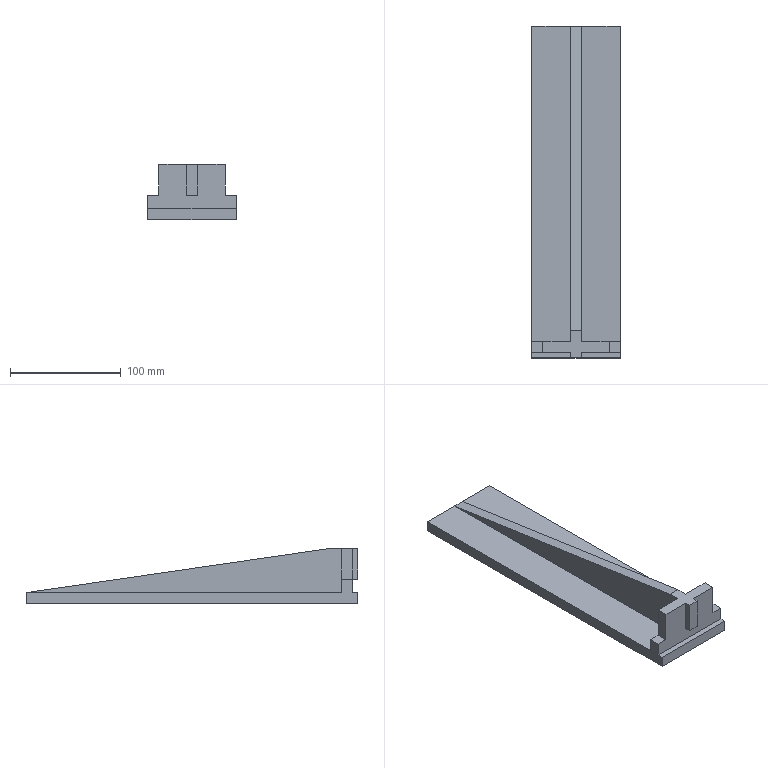Part | STEP file | duizhongban | 1 solid | 23 faces | box 80 x 300 x 50 mm | volume 326800 mm3 | plane 23